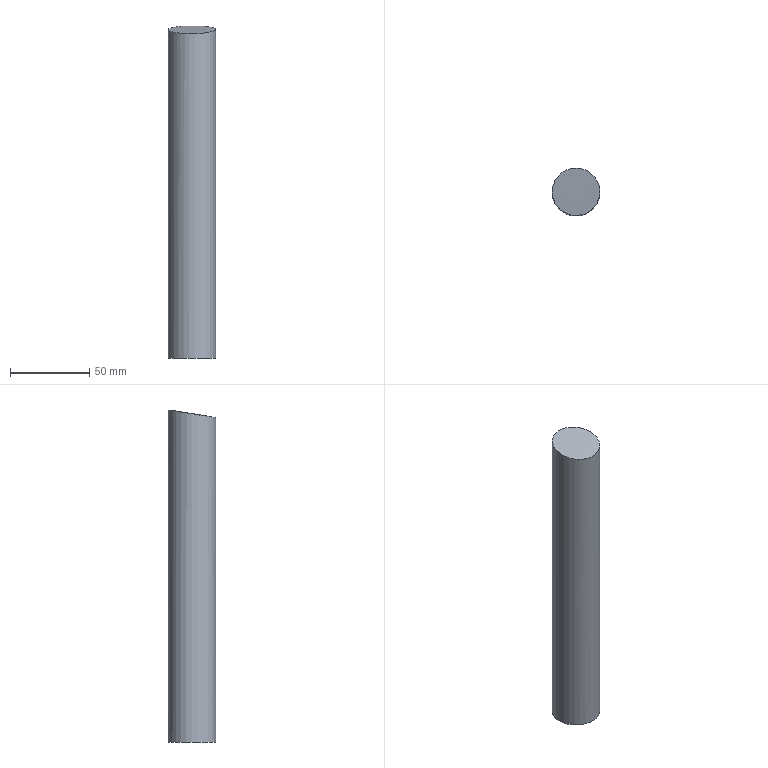Part | NX | features solid 2 | 1 solid | 3 faces | box 30 x 30 x 209.476 mm | volume 146403 mm3 | cylinder 1 | spline 1 | plane 1 | commonest cylinder face diameters 30 x1
STEP:
#1=CARTESIAN_POINT('',(293.789,-549.966,77.443));
#2=VERTEX_POINT('',#1);
#3=CARTESIAN_POINT('',(298.31,-553.864,76.782));
#4=CARTESIAN_POINT('',(291.873,-549.008,77.608));
#5=CARTESIAN_POINT('',(288.432,-539.101,79.262));
#6=CARTESIAN_POINT('',(293.846,-527.671,81.037));
#7=CARTESIAN_POINT('',(305.915,-523.371,81.712));
#8=CARTESIAN_POINT('',(317.451,-528.981,80.971));
#9=CARTESIAN_POINT('',(321.566,-540.934,79.143));
#10=CARTESIAN_POINT('',(317.047,-550.4,77.499));
#11=CARTESIAN_POINT('',(310.138,-554.511,76.729));
#12=CARTESIAN_POINT('',(304.151,-555.372,76.541));
#13=CARTESIAN_POINT('',(298.31,-553.864,76.782));
#14=CARTESIAN_POINT('',(291.873,-549.008,77.608));
#15=CARTESIAN_POINT('',(288.432,-539.101,79.262));
#16=B_SPLINE_CURVE_WITH_KNOTS('',3,(#3,#4,#5,#6,#7,#8,#9,#10,#11,#12,#13,#14,#15),.UNSPECIFIED.,.T.,.F.,(1,1,1,1,1,1,1,1,1,1,1,1,1,1,1,1,1),(-0.0177,-0.0118,-0.005899,0.,0.0118,0.0236,0.03539,0.04719,0.05899,0.07079,0.07669,0.08259,0.08849,0.09438,0.1062,0.118,0.1298),.UNSPECIFIED.);
#17=EDGE_CURVE('',#2,#2,#16,.T.);
#18=ORIENTED_EDGE('',*,*,#17,.T.);
#19=EDGE_LOOP('',(#18));
#20=FACE_BOUND('',#19,.T.);
#21=CARTESIAN_POINT('',(320.,-540.,-128.));
#22=VERTEX_POINT('',#21);
#23=CARTESIAN_POINT('',(305.,-540.,-128.));
#24=DIRECTION('',(0.,0.,1.));
#25=DIRECTION('',(1.,0.,0.));
#26=AXIS2_PLACEMENT_3D('',#23,#24,#25);
#27=CIRCLE('',#26,15.);
#28=EDGE_CURVE('',#22,#22,#27,.F.);
#29=ORIENTED_EDGE('',*,*,#28,.F.);
#30=EDGE_LOOP('',(#29));
#31=FACE_BOUND('',#30,.T.);
#32=CARTESIAN_POINT('',(305.,-540.,-28.));
#33=DIRECTION('',(0.,0.,-1.));
#34=DIRECTION('',(0.,1.,0.));
#35=AXIS2_PLACEMENT_3D('',#32,#33,#34);
#36=CYLINDRICAL_SURFACE('',#35,15.);
#37=ADVANCED_FACE('',(#20,#31),#36,.T.);
#38=ORIENTED_EDGE('',*,*,#17,.F.);
#39=EDGE_LOOP('',(#38));
#40=FACE_BOUND('',#39,.T.);
#41=CARTESIAN_POINT('',(320.265,-555.158,76.664));
#42=CARTESIAN_POINT('',(310.095,-555.191,76.607));
#43=CARTESIAN_POINT('',(299.926,-555.224,76.546));
#44=CARTESIAN_POINT('',(289.756,-555.257,76.483));
#45=CARTESIAN_POINT('',(320.264,-545.013,78.49));
#46=CARTESIAN_POINT('',(310.095,-545.055,78.431));
#47=CARTESIAN_POINT('',(299.926,-545.097,78.37));
#48=CARTESIAN_POINT('',(289.756,-545.139,78.305));
#49=CARTESIAN_POINT('',(320.264,-534.841,80.137));
#50=CARTESIAN_POINT('',(310.095,-534.892,80.077));
#51=CARTESIAN_POINT('',(299.926,-534.943,80.015));
#52=CARTESIAN_POINT('',(289.756,-534.994,79.95));
#53=CARTESIAN_POINT('',(320.264,-524.639,81.606));
#54=CARTESIAN_POINT('',(310.095,-524.7,81.546));
#55=CARTESIAN_POINT('',(299.925,-524.76,81.484));
#56=CARTESIAN_POINT('',(289.756,-524.82,81.418));
#57=B_SPLINE_SURFACE_WITH_KNOTS('',3,3,((#41,#42,#43,#44),(#45,#46,#47,#48),(#49,#50,#51,#52),(#53,#54,#55,#56)),.UNSPECIFIED.,.F.,.F.,.F.,(4,4),(4,4),(0.208,0.3758),(0.3972,0.5451),.UNSPECIFIED.);
#58=ADVANCED_FACE('',(#40),#57,.T.);
#59=ORIENTED_EDGE('',*,*,#28,.T.);
#60=EDGE_LOOP('',(#59));
#61=FACE_BOUND('',#60,.T.);
#62=CARTESIAN_POINT('',(305.,-540.,-128.));
#63=DIRECTION('',(0.,0.,1.));
#64=DIRECTION('',(0.,-1.,0.));
#65=AXIS2_PLACEMENT_3D('',#62,#63,#64);
#66=PLANE('',#65);
#67=ADVANCED_FACE('',(#61),#66,.F.);
#68=CLOSED_SHELL('',(#37,#58,#67));
#69=MANIFOLD_SOLID_BREP('',#68);
#70=(LENGTH_UNIT()NAMED_UNIT(*)SI_UNIT(.MILLI.,.METRE.));
#71=UNCERTAINTY_MEASURE_WITH_UNIT(LENGTH_MEASURE(0.0508),#70,'','');
#72=(NAMED_UNIT(*)PLANE_ANGLE_UNIT()SI_UNIT($,.RADIAN.));
#73=(NAMED_UNIT(*)SI_UNIT($,.STERADIAN.)SOLID_ANGLE_UNIT());
#74=(GEOMETRIC_REPRESENTATION_CONTEXT(3)GLOBAL_UNCERTAINTY_ASSIGNED_CONTEXT((#71))GLOBAL_UNIT_ASSIGNED_CONTEXT((#70,#72,#73))REPRESENTATION_CONTEXT('',''));
#75=ADVANCED_BREP_SHAPE_REPRESENTATION('',(#69),#74);